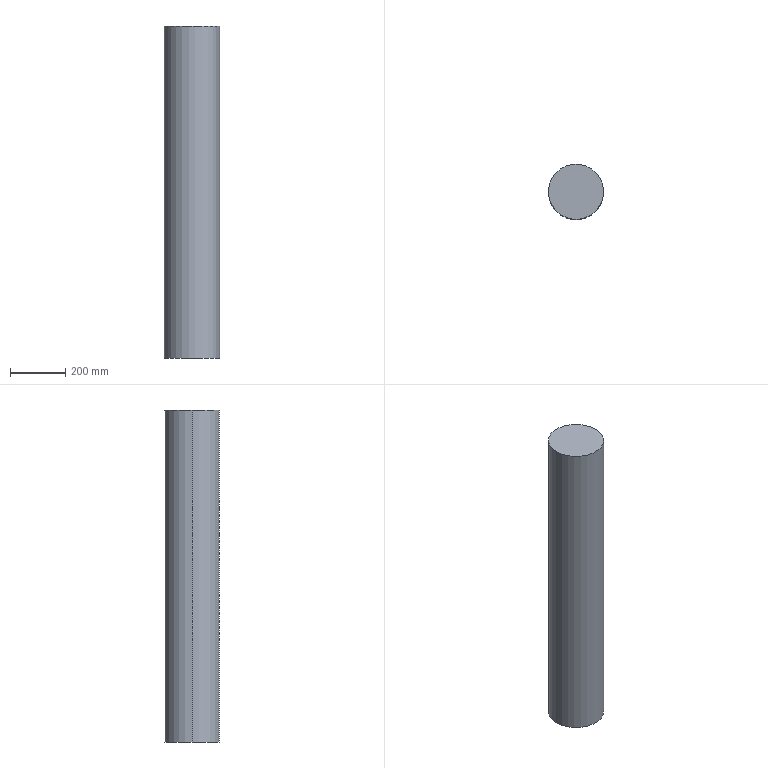Part | SolidWorks | features Extrusion 1 | 1 solid | 4 faces | box 200 x 200 x 1200 mm | volume 37699112 mm3 | cylinder 2 | plane 2 | commonest cylinder face diameters 200 x2
STEP:
#1=CARTESIAN_POINT('',(100.,0.,1200.));
#2=VERTEX_POINT('',#1);
#3=CARTESIAN_POINT('',(-100.,0.,1200.));
#4=VERTEX_POINT('',#3);
#5=CARTESIAN_POINT('',(0.,0.,1200.));
#6=DIRECTION('',(0.,0.,1.));
#7=DIRECTION('',(1.,0.,0.));
#8=AXIS2_PLACEMENT_3D('',#5,#6,#7);
#9=CIRCLE('',#8,100.);
#10=EDGE_CURVE('',#2,#4,#9,.T.);
#11=ORIENTED_EDGE('',*,*,#10,.F.);
#12=CARTESIAN_POINT('',(100.,0.,0.));
#13=VERTEX_POINT('',#12);
#14=CARTESIAN_POINT('',(100.,0.,1200.));
#15=DIRECTION('',(0.,0.,-1.));
#16=VECTOR('',#15,1000.);
#17=LINE('',#14,#16);
#18=EDGE_CURVE('',#2,#13,#17,.T.);
#19=ORIENTED_EDGE('',*,*,#18,.T.);
#20=CARTESIAN_POINT('',(-100.,0.,0.));
#21=VERTEX_POINT('',#20);
#22=CARTESIAN_POINT('',(0.,0.,0.));
#23=DIRECTION('',(0.,0.,1.));
#24=DIRECTION('',(1.,0.,0.));
#25=AXIS2_PLACEMENT_3D('',#22,#23,#24);
#26=CIRCLE('',#25,100.);
#27=EDGE_CURVE('',#13,#21,#26,.T.);
#28=ORIENTED_EDGE('',*,*,#27,.T.);
#29=CARTESIAN_POINT('',(-100.,0.,1200.));
#30=DIRECTION('',(0.,0.,-1.));
#31=VECTOR('',#30,1000.);
#32=LINE('',#29,#31);
#33=EDGE_CURVE('',#4,#21,#32,.T.);
#34=ORIENTED_EDGE('',*,*,#33,.F.);
#35=EDGE_LOOP('',(#11,#19,#28,#34));
#36=FACE_OUTER_BOUND('',#35,.T.);
#37=CARTESIAN_POINT('',(0.,0.,1200.));
#38=DIRECTION('',(0.,0.,-1.));
#39=DIRECTION('',(-1.,0.,0.));
#40=AXIS2_PLACEMENT_3D('',#37,#38,#39);
#41=CYLINDRICAL_SURFACE('',#40,100.);
#42=ADVANCED_FACE('',(#36),#41,.T.);
#43=ORIENTED_EDGE('',*,*,#18,.F.);
#44=CARTESIAN_POINT('',(0.,0.,1200.));
#45=DIRECTION('',(0.,0.,1.));
#46=DIRECTION('',(1.,0.,0.));
#47=AXIS2_PLACEMENT_3D('',#44,#45,#46);
#48=CIRCLE('',#47,100.);
#49=EDGE_CURVE('',#4,#2,#48,.T.);
#50=ORIENTED_EDGE('',*,*,#49,.F.);
#51=ORIENTED_EDGE('',*,*,#33,.T.);
#52=CARTESIAN_POINT('',(0.,0.,0.));
#53=DIRECTION('',(0.,0.,1.));
#54=DIRECTION('',(1.,0.,0.));
#55=AXIS2_PLACEMENT_3D('',#52,#53,#54);
#56=CIRCLE('',#55,100.);
#57=EDGE_CURVE('',#21,#13,#56,.T.);
#58=ORIENTED_EDGE('',*,*,#57,.T.);
#59=EDGE_LOOP('',(#43,#50,#51,#58));
#60=FACE_OUTER_BOUND('',#59,.T.);
#61=CARTESIAN_POINT('',(0.,0.,1200.));
#62=DIRECTION('',(0.,0.,-1.));
#63=DIRECTION('',(-1.,0.,0.));
#64=AXIS2_PLACEMENT_3D('',#61,#62,#63);
#65=CYLINDRICAL_SURFACE('',#64,100.);
#66=ADVANCED_FACE('',(#60),#65,.T.);
#67=ORIENTED_EDGE('',*,*,#49,.T.);
#68=ORIENTED_EDGE('',*,*,#10,.T.);
#69=EDGE_LOOP('',(#67,#68));
#70=FACE_OUTER_BOUND('',#69,.T.);
#71=CARTESIAN_POINT('',(0.,0.,1200.));
#72=DIRECTION('',(0.,0.,1.));
#73=DIRECTION('',(1.,0.,0.));
#74=AXIS2_PLACEMENT_3D('',#71,#72,#73);
#75=PLANE('',#74);
#76=ADVANCED_FACE('',(#70),#75,.T.);
#77=ORIENTED_EDGE('',*,*,#57,.F.);
#78=ORIENTED_EDGE('',*,*,#27,.F.);
#79=EDGE_LOOP('',(#77,#78));
#80=FACE_OUTER_BOUND('',#79,.T.);
#81=CARTESIAN_POINT('',(0.,0.,0.));
#82=DIRECTION('',(0.,0.,1.));
#83=DIRECTION('',(1.,0.,0.));
#84=AXIS2_PLACEMENT_3D('',#81,#82,#83);
#85=PLANE('',#84);
#86=ADVANCED_FACE('',(#80),#85,.F.);
#87=CLOSED_SHELL('',(#42,#66,#76,#86));
#88=MANIFOLD_SOLID_BREP('',#87);
#89=CARTESIAN_POINT('',(0.,0.,0.));
#90=DIRECTION('',(0.,0.,1.));
#91=DIRECTION('',(1.,0.,0.));
#92=AXIS2_PLACEMENT_3D('',#89,#90,#91);
#93=(LENGTH_UNIT()NAMED_UNIT(*)SI_UNIT(.MILLI.,.METRE.));
#94=UNCERTAINTY_MEASURE_WITH_UNIT(LENGTH_MEASURE(0.00001),#93,'','');
#95=(NAMED_UNIT(*)PLANE_ANGLE_UNIT()SI_UNIT($,.RADIAN.));
#96=(NAMED_UNIT(*)SI_UNIT($,.STERADIAN.)SOLID_ANGLE_UNIT());
#97=(GEOMETRIC_REPRESENTATION_CONTEXT(3)GLOBAL_UNCERTAINTY_ASSIGNED_CONTEXT((#94))GLOBAL_UNIT_ASSIGNED_CONTEXT((#93,#95,#96))REPRESENTATION_CONTEXT('',''));
#98=ADVANCED_BREP_SHAPE_REPRESENTATION('',(#88,#92),#97);